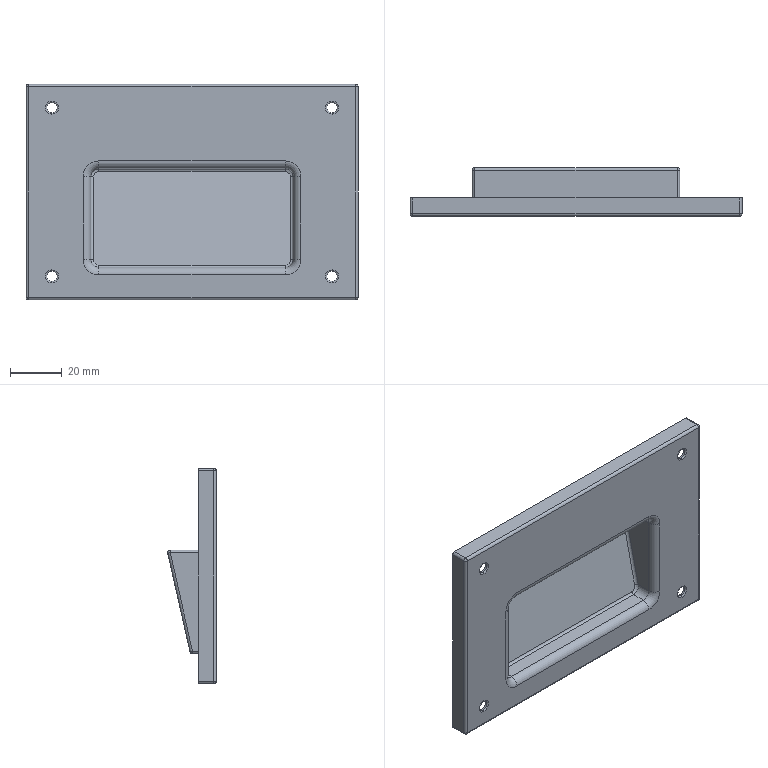Part | SolidWorks | features Cut 3, Fillet 3, Boss 1, Extrusion 1 | 1 solid | 101 faces | box 128 x 18.75 x 83 mm | volume 17902 mm3 | cylinder 48 | plane 21 | torus 16 | sphere 12 | spline 4 | commonest cylinder face diameters 2 x32 4 x8 6 x8